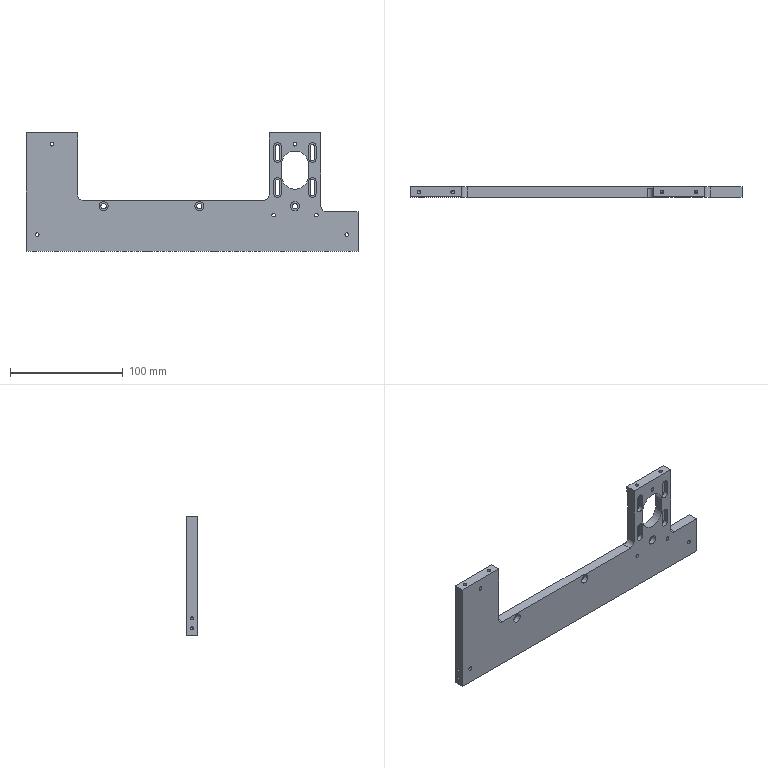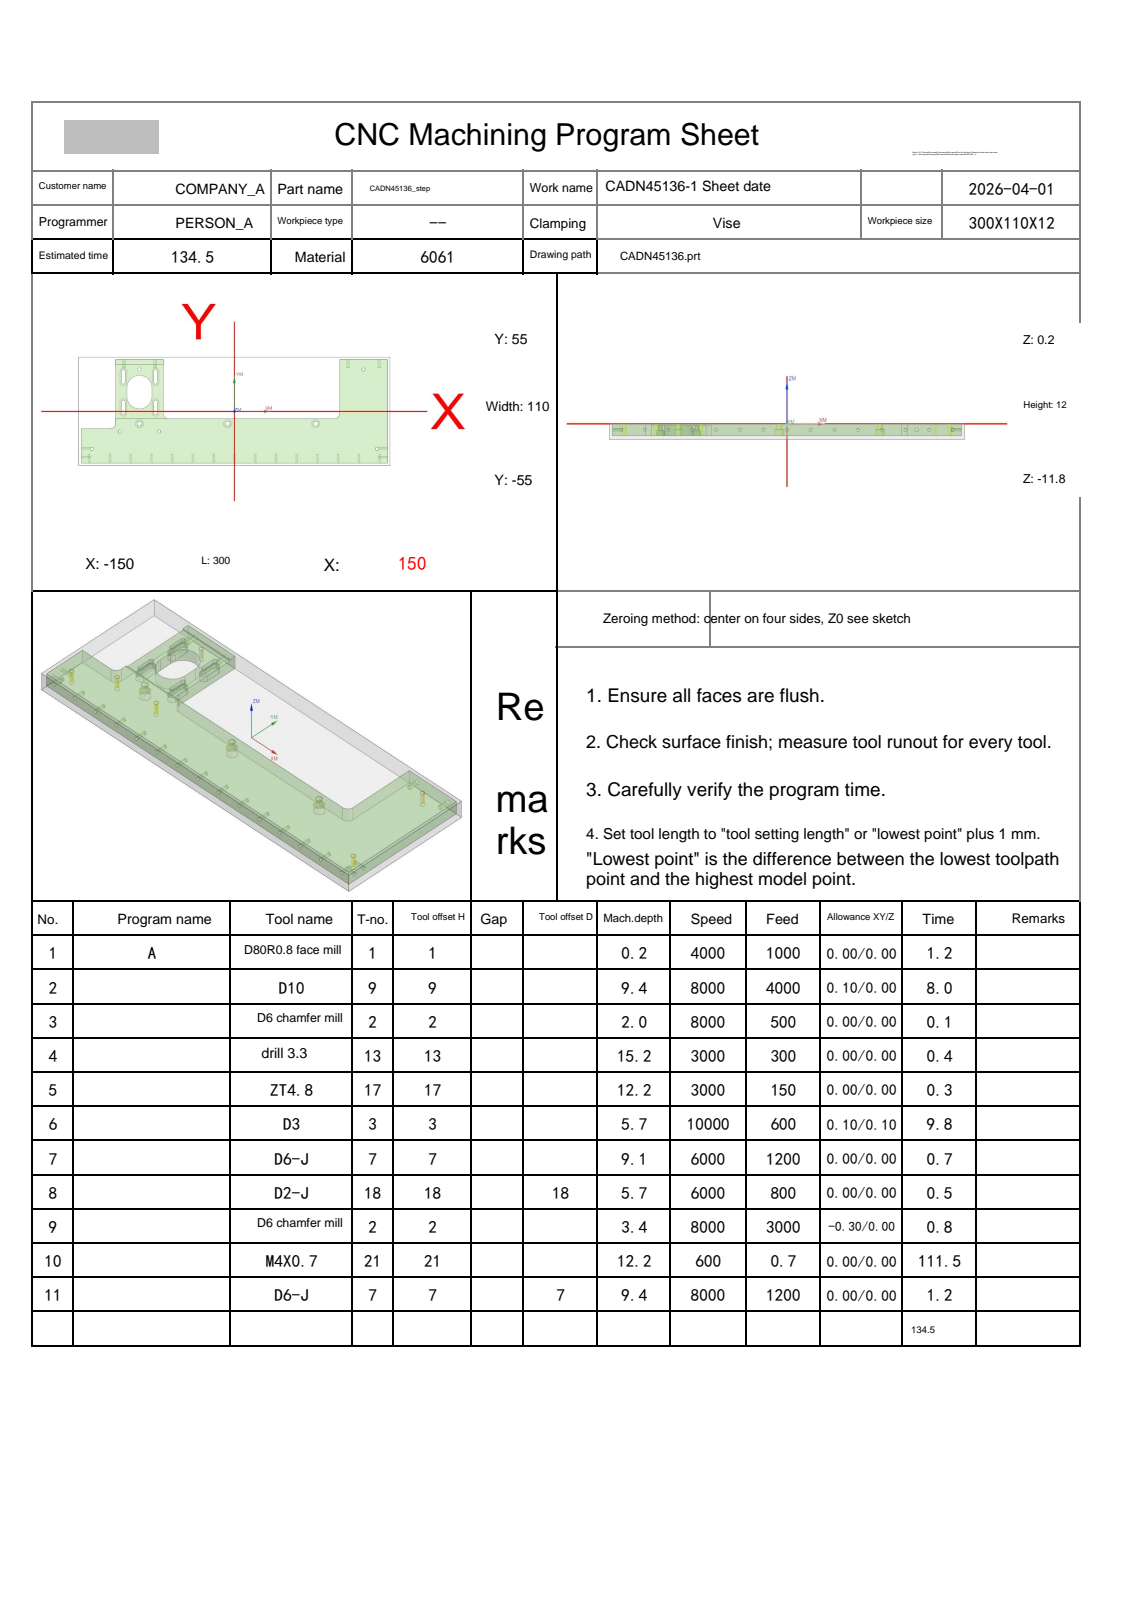NC program | NX | posted by the shop | part box 295 x 9 x 105 mm
Lines 40 to 820 of 7463:
N2 T09 M06
(D10  D=10. R=0. H=09 ce=0.25 di=0.10)
G00 G90 G54 X-68.786 Y65.963 M03 S8000
G43 H09 Z20.
M08
Z-7.2
G01 X-68.771 Y65.864 Z-7.825 F4000.
X-68.756 Y65.765 Z-8.072
X-68.741 Y65.666 Z-8.254
X-68.727 Y65.567 Z-8.4
X-68.712 Y65.468 Z-8.523
X-68.697 Y65.369 Z-8.628
X-68.683 Y65.271 Z-8.72
X-68.668 Y65.172 Z-8.8
X-68.653 Y65.073 Z-8.87
X-68.638 Y64.974 Z-8.932
X-68.624 Y64.875 Z-8.986
X-68.609 Y64.776 Z-9.033
X-68.594 Y64.677 Z-9.074
X-68.579 Y64.578 Z-9.108
X-68.565 Y64.479 Z-9.136
X-68.55 Y64.38 Z-9.16
X-68.535 Y64.281 Z-9.177
X-68.52 Y64.183 Z-9.19
X-68.506 Y64.084 Z-9.197
X-68.491 Y63.985 Z-9.2
X-68.183 Y61.92
G03 X-67.828 Y61.51 I.503 J.077
X-64.07 Y61.003 I3.766 J13.735
X-55.015 Y60.895 I9.055 J380.264
X-53.111 Y60.9 I0.0 J380.372
G01 X148.548 Y60.876
G02 X154.516 Y56.713 I-.244 J-6.709
X155.74 Y50.873 I-15.367 J-6.267
X155.919 Y41.406 I-249.458 J-9.468
X155.9 Y38.276 I-249.637 J0.0
G01 X155.881 Y-53.443
G02 X151.609 Y-59.576 I-6.76 J.154
X145.818 Y-60.747 I-6.194 J15.737
X136.002 Y-60.92 I-9.816 J277.475
X132.62 Y-60.9 I0.0 J277.648
G01 X-148.443 Y-60.881
G02 X-154.576 Y-56.609 I.154 J6.761
X-155.75 Y-50.758 I15.84 J6.222
X-155.919 Y-40.968 I283.441 J9.79
X-155.9 Y-37.62 I283.61 J0.0
G01 X-155.881 Y53.463
G02 X-151.482 Y59.632 I6.792 J-.189
X-145.858 Y60.744 I6.093 J-16.036
X-136.388 Y60.919 I9.47 J-257.302
X-133.261 Y60.9 I0.0 J-257.476
G01 X-70.041 Y60.879
G03 X-57.209 Y60.291 I12.832 J139.682
X-55.325 Y60.304 I0.0 J140.271
G01 X146.849 Y60.277
G02 X153.44 Y55.91 I-.376 J-7.725
X155.033 Y49.733 I-14.85 J-7.123
X155.315 Y40.999 I-135.175 J-8.734
X155.297 Y38.82 I-135.457 J0.0
G01 X155.276 Y-51.847
G02 X150.921 Y-58.441 I-7.715 J.36
X144.799 Y-60.029 I-7.08 J14.703
X136.255 Y-60.312 I-8.544 J128.757
X134.246 Y-60.297 I0.0 J129.04
G01 X-146.788 Y-60.279
G02 X-153.493 Y-55.822 I.313 J7.744
X-155.023 Y-49.865 I14.84 J6.985
X-155.302 Y-41.99 I110.955 J7.875
X-155.294 Y-40.632 I111.234 J0.0
G01 X-155.279 Y51.788
G02 X-150.981 Y58.41 I7.703 J-.294
X-144.864 Y60.023 I7.093 J-14.49
X-136.955 Y60.303 I7.909 J-111.65
X-135.571 Y60.294 I0.0 J-111.93
G01 X-71.631 Y60.284
G03 X-62.812 Y59.814 I57.469 J996.395
X-51.581 Y59.699 I11.231 J545.885
X-50.111 Y59.701 I0.0 J546.001
G01 X145.169 Y59.68
G02 X152.839 Y54.507 I-.295 J-8.712
X154.414 Y48.069 I-16.783 J-7.517
X154.705 Y39.47 I-126.982 J-8.599
X154.694 Y37.816 I-127.273 J0.0
G01 X154.675 Y-50.243
G02 X149.608 Y-57.796 I-8.677 J.345
X143.065 Y-59.417 I-7.586 J16.605
X133.778 Y-59.715 I-9.287 J144.477
X131.492 Y-59.697 I0.0 J144.775
G01 X-145.208 Y-59.677
G02 X-152.851 Y-54.498 I.321 J8.702
X-154.412 Y-48.122 I16.765 J7.484
X-154.706 Y-39.479 I126.879 J8.643
X-154.695 Y-37.809 I127.173 J0.0
G01 X-154.675 Y50.251
G02 X-149.622 Y57.786 I8.675 J-.355
X-143.195 Y59.404 I7.576 J-16.526
X-134.131 Y59.712 I9.064 J-132.923
X-132.042 Y59.696 I0.0 J-133.231
G01 X-72.722 Y59.682
G02 X-63.107 Y59.239 I-33.813 J-837.622
G03 X-51.393 Y59.1 I11.714 J493.752
X-50.11 Y59.101 I0.0 J493.891
G01 X143.669 Y59.077
G02 X148.675 Y57.598 I-.315 J-10.277
X150.125 Y57.047 I-1.928 J-7.251
G01 X151.212 Y56.212
X152.047 Y55.125
G02 X153.419 Y50.239 I-16.938 J-7.393
X154.07 Y41.14 I-63.251 J-9.099
X154.067 Y40.491 I-63.902 J0.0
G01 X154.099 Y30.351
X154.076 Y-48.649
G02 X152.605 Y-53.654 I-9.869 J.182
X152.047 Y-55.125 I-7.571 J2.033
G01 X151.212 Y-56.212
X150.125 Y-57.047
G02 X145.652 Y-58.348 I-7.112 J16.105
X136.776 Y-59.053 I-8.875 J55.541
G01 X136.51 Y-59.052
X125.35 Y-59.099
X-143.67 Y-59.075
G02 X-148.676 Y-57.599 I.237 J10.028
X-150.125 Y-57.047 I2.048 J7.549
G01 X-151.212 Y-56.212
X-152.047 Y-55.125
G02 X-153.391 Y-50.416 I16.58 J7.279
X-154.066 Y-41.352 I60.501 J9.065
X-154.063 Y-40.79 I61.176 J0.0
G01 X-154.098 Y-31.671
X-154.076 Y48.649
G02 X-148.384 Y57.183 I9.462 J-.146
X-141.53 Y58.809 I8.014 J-18.516
X-132.244 Y59.109 I9.286 J-143.8
X-130.257 Y59.095 I0.0 J-144.1
G01 X-73.577 Y59.08
G02 X-62.877 Y58.642 I-27.703 J-807.761
G03 X-50.397 Y58.5 I12.48 J549.906
X-49.15 Y58.502 I0.0 J550.047
G01 X142.169 Y58.479
G02 X146.239 Y57.75 I-.385 J-13.872
X146.807 Y57.765 I.568 J-10.591
X148.751 Y57.585 I0.0 J-10.606
G03 X146.437 Y57.771 I-2.314 J-14.306
X145.781 Y57.756 I0.0 J-14.492
X137.77 Y58.028 I-8.011 J-117.995
X136.203 Y58.018 I0.0 J-118.266
G01 X-56.084 Y58.043
G02 X-72.109 Y58.552 I6.852 J468.627
G03 X-80.688 Y58.618 I-8.844 J-591.068
G01 X-134.548 Y58.59
G03 X-135.199 Y58.593 I-.651 J-60.006
X-143.402 Y58.03 I0.0 J-60.01
X-149.644 Y55.55 I1.793 J-13.612
X-153.206 Y49.151 I6.171 J-7.625
X-153.61 Y42.924 I47.678 J-6.227
X-153.603 Y42.089 I48.083 J0.0
G01 X-153.598 Y-39.071
G03 X-153.602 Y-39.931 I77.983 J-.86
X-153.086 Y-48.891 I77.988 J0.0
G01 X-152.75 Y-50.863
G03 X-152.774 Y-51.633 I12.285 J-.77
X-152.571 Y-53.859 I12.309 J0.0
G02 X-152.774 Y-51.633 I12.106 J2.226
X-152.75 Y-50.863 I12.309 J0.0
G03 X-152.949 Y-41.559 I-232.624 J-.324
G02 X-153.024 Y-31.151 I719.15 J10.408
X-153.018 Y-28.119 I719.225 J0.0
G01 X-152.994 Y42.301
G02 X-153. Y42.949 I35.009 J.649
X-152.496 Y48.871 I35.015 J0.0
X-146.142 Y56.306 I9.945 J-2.067
X-138.997 Y57.773 I8.169 J-21.648
X-129.006 Y58.032 I9.991 J-192.317
X-126.522 Y58.016 I0.0 J-192.577
G01 X-75.182 Y57.996
G02 X-61.404 Y57.536 I-23.436 J-909.651
G03 X-48.423 Y57.418 I12.981 J712.896
X-46.331 Y57.421 I0.0 J713.014
G01 X99.827 Y57.444
X100.141 Y57.571
X101.502 Y57.75
X145.962
G03 X146.462 Y58.25 I0.0 J.5
X146.23 Y58.672 I-.5 J0.0
G01 X145.472 Y59.154
X143.803 Y60.216 Z-9.1
X143.471 Y60.426
X143.41 Y60.46
X143.345 Y60.484
X143.277 Y60.499
X143.207 Y60.504
X101.792 Y60.822
X101.709 Y60.816
X101.628 Y60.795
X101.551 Y60.762
X101.481 Y60.717
X101.42 Y60.66
X101.369 Y60.594
X101.329 Y60.521
X101.202 Y60.227
X100.415 Y58.412 Z-9.2
X100.076 Y57.643
G02 X99.194 Y57.273 I-.934 J.987
X94.052 Y56.951 I-5.142 J40.964
X93.238 Y56.959 I0.0 J41.286
G01 X-54.412 Y56.957
G02 X-66.375 Y57.254 I1.4 J298.37
G01 X-67.141 Y57.571
X-68.498 Y57.75
X-114.559 Y57.742
G02 X-121.715 Y57.521 I-7.155 J115.808
X-123.687 Y57.538 I0.0 J116.029
G03 X-126.982 Y57.558 I-3.295 J-268.593
X-137.903 Y57.336 I0.0 J-268.613
X-145.133 Y56.003 I.793 J-24.574
X-151.833 Y48.166 I3.59 J-9.852
X-152.494 Y41.412 I34.197 J-6.754
X-152.493 Y41.13 I34.857 J0.0
G01 X-152.538 Y31.59
X-152.56 Y-16.114
X-152.75 Y-17.498
Y-47.858
G02 X-153.25 Y-48.358 I-.5 J0.0
X-153.672 Y-48.126 I0.0 J.5
G01 X-154.155 Y-47.366
X-155.216 Y-45.696 Z-9.1
X-155.427 Y-45.364
X-155.46 Y-45.303
X-155.484 Y-45.239
X-155.499 Y-45.172
X-155.505 Y-45.104
X-155.934 Y-18.062
X-155.928 Y-17.978
X-155.908 Y-17.896
X-155.875 Y-17.819
X-155.829 Y-17.748
X-155.772 Y-17.686
X-155.706 Y-17.635
X-155.632 Y-17.595
X-155.242 Y-17.426
X-153.425 Y-16.642 Z-9.2
X-152.755 Y-16.346
G03 X-152.322 Y-15.277 I-1.299 J1.149
X-151.955 Y-9.758 I-41.263 J5.519
X-151.962 Y-9.007 I-41.63 J0.0
G01 X-151.911 Y39.449
G02 X-151.915 Y40.07 I41.231 J.621
X-151.343 Y46.917 I41.235 J0.0
X-144.116 Y55.353 I10.759 J-1.903
X-136.649 Y56.725 I8.369 J-24.555
X-125.37 Y56.959 I11.279 J-271.073
X-122.371 Y56.942 I0.0 J-271.308
G03 X-121.606 Y56.939 I.764 J93.639
X-117.125 Y57.047 I0.0 J93.642
G01 X-115.859 Y57.571
X-114.55 Y57.743
X-115.859 Y57.571
G02 X-119.804 Y56.605 I-4.069 J8.073
X-130.792 Y56.413 I-10.988 J314.503
G01 X-131.508
X-131.837 Y56.414
G03 X-140.295 Y55.769 I0.0 J-55.728
X-146.815 Y53.03 I2.081 J-14.085
X-150.712 Y46.343 I7.555 J-8.882
X-151.412 Y39.014 I38.02 J-7.329
X-151.411 Y38.708 I38.72 J0.0
G01 X-151.458 Y28.808
X-151.485 Y-8.765
G02 X-151.481 Y-9.31 I-40.224 J-.545
X-151.821 Y-14.533 I-40.228 J0.0
G03 X-152.506 Y-15.984 I4.769 J-3.138
G02 X-151.728 Y-14.401 I5.56 J-1.751
G03 X-151.04 Y-10.594 I-11.607 J4.064
X-150.851 Y-2.255 I-183.773 J8.339
X-150.859 Y-.53 I-183.962 J0.0
G01 X-150.832 Y36.809
G02 X-150.837 Y37.511 I48.195 J.702
X-150.261 Y44.939 I48.2 J0.0
X-146.631 Y51.841 I11.812 J-1.807
X-139.977 Y54.993 I9.229 J-10.884
X-131.236 Y55.792 I8.741 J-47.384
G01 X-131.146
G03 X-120.479 Y56.007 I-.823 J305.744
X-117.968 Y56.4 I-.168 J9.294
G01 X-117.125 Y57.047
G02 X-119.928 Y55.776 I-3.254 J3.449
X-126.122 Y55.388 I-6.194 J49.27
X-126.459 Y55.389 I0.0 J49.658
G03 X-126.977 Y55.39 I-.518 J-111.012
X-136.698 Y54.964 I0.0 J-111.013
X-143.704 Y53.001 I1.554 J-19.027
X-149.377 Y45.566 I5.649 J-10.193
X-150.291 Y38.08 I31.407 J-7.633
X-150.378 Y27.767 I609.102 J-10.313
G01 Y26.86
X-150.403 Y-5.23
G02 X-150.398 Y-5.905 I-49.547 J-.675
X-150.828 Y-12.419 I-49.552 J0.0
X-151.212 Y-13.788 I-4.983 J.66
G01 X-151.87 Y-14.645
G03 X-150.747 Y-12.973 I-5.022 J4.588
X-149.95 Y-8.12 I-16.475 J5.196
X-149.765 Y1.489 I-248.778 J9.609
X-149.778 Y4.089 I-248.964 J0.0
G01 X-149.748 Y34.849
G02 X-149.752 Y35.499 I50.631 J.65
X-149.142 Y43.337 I50.635 J0.0
X-145.752 Y50.231 I12.711 J-1.969
X-138.839 Y53.806 I9.685 J-10.257
X-130.019 Y54.701 I8.98 J-44.607
G03 X-121.432 Y55.052 I-.675 J121.785
X-118.603 Y55.728 I-.487 J8.287
G02 X-117.974 Y56.395 I2.464 J-1.694
G03 X-118.614 Y55.697 I1.576 J-2.088
G02 X-121.316 Y54.754 I-3.37 J5.308
X-128.025 Y54.283 I-7.13 J53.574
G03 X-136.933 Y53.617 I.376 J-64.906
X-143.797 Y50.919 I2.195 J-15.669
X-148.345 Y43.737 I7.694 J-9.903
X-149.217 Y35.941 I35.474 J-7.913
X-149.297 Y25.914 I621.652 J-10.028
G01 Y25.622
X-149.325 Y-2.828
G02 X-149.321 Y-3.477 I-55.604 J-.648
X-149.792 Y-10.702 I-55.608 J0.0
X-150.65 Y-13.348 I-7.16 J.858
G01 X-151.205 Y-13.782
G03 X-149.699 Y-11.683 I-1.87 J2.932
X-148.861 Y-5.993 I-21.722 J6.106
X-148.684 Y4.381 I-305.289 J10.374
X-148.698 Y7.269 I-305.465 J0.0
G01 X-148.668 Y32.809
G02 X-148.672 Y33.485 I54.884 J.676
X-148.061 Y41.658 I54.888 J0.0
X-144.879 Y48.622 I13.632 J-2.018
X-137.852 Y52.591 I10.07 J-9.624
X-129.468 Y53.604 I9.193 J-40.884
G03 X-121.979 Y54.13 I-1.305 J72.255
X-119.154 Y54.999 I-.943 J8.088
G01 X-118.572 Y55.744
G02 X-119.554 Y54.67 I-3.103 J1.85
X-123.255 Y53.599 I-4.607 J8.991
X-130.947 Y53.035 I-12.623 J119.535
G03 X-138.788 Y51.686 I1.192 J-30.378
X-147.067 Y42.897 I3.873 J-11.942
X-148.097 Y35.245 I31.408 J-8.123
X-148.226 Y24.802 I424.702 J-10.443
X-148.218 Y22.226 I424.83 J0.0
G01 X-148.248 Y-.905
G02 X-148.244 Y-1.559 I-58.96 J-.654
X-148.78 Y-9.488 I-58.964 J0.0
X-149.931 Y-12.826 I-8.323 J1.003
G01 X-150.601 Y-13.319
G03 X-149.613 Y-12.538 I-3.219 J5.094
X-148.285 Y-9.065 I-6.834 J4.603
X-147.671 Y-1.149 I-50.739 J7.916
G01 Y-.93
X-147.618 Y9.309
X-147.589 Y30.809
G02 X-147.593 Y31.447 I61.772 J.638
X-147.028 Y39.783 I61.776 J0.0
X-144.168 Y46.821 I14.934 J-1.968
X-137.126 Y51.308 I10.493 J-8.698
X-129.132 Y52.509 I9.654 J-37.075
G03 X-122.251 Y53.253 I-2.097 J51.6
X-119.385 Y54.43 I-1.105 J6.767
X-119.047 Y55.125 I-2.527 J1.662
G02 X-120.426 Y53.615 I-2.203 J.628
X-125.058 Y52.432 I-5.836 J13.182
G03 X-132.691 Y51.659 I52.124 J-553.045
X-139.938 Y49.455 I2.129 J-20.019
X-145.982 Y41.424 I6.51 J-11.19
X-147.031 Y33.17 I34.13 J-8.53
X-147.139 Y22.944 I486.902 J-10.226
X-147.137 Y21.831 I487.009 J0.0
G01 X-147.168 Y1.013
G02 X-147.164 Y.337 I-65.753 J-.676
X-147.728 Y-8.252 I-65.757 J0.0
X-149.106 Y-12.263 I-9.883 J1.154
X-150.025 Y-12.912 I-1.278 J.835
G03 X-148.319 Y-11.362 I-.853 J2.653
X-147.013 Y-6.549 I-12.819 J6.062
X-146.552 Y2.684 I-92.147 J9.233
X-146.556 Y3.578 I-92.609 J0.0
G01 X-146.499 Y29.789
G02 X-146.502 Y30.295 I55.704 J.506
X-145.837 Y38.874 I55.706 J0.0
X-142.562 Y46.118 I14.6 J-2.238
X-135.397 Y50.326 I10.589 J-9.827
X-128.536 Y51.453 I10.344 J-41.506
G03 X-122.21 Y52.459 I-2.581 J36.644
X-119.615 Y53.792 I-1.442 J5.999
G01 X-119.293 Y54.531
G02 X-120.933 Y52.701 I-2.73 J.796
X-125.878 Y51.343 I-6.657 J14.559
G03 X-133.252 Y50.271 I14.392 J-124.874
X-140.401 Y47.159 I2.877 J-16.377
X-144.992 Y39.65 I8.849 J-10.568
X-145.952 Y31.503 I37.313 J-8.529
X-146.08 Y16.182 I919.511 J-15.321
X-146.058 Y9.78 I919.639 J0.0
G02 X-146.039 Y6.984 I-211.212 J-2.796
X-146.331 Y-4.12 I-211.23 J0.0
X-147.448 Y-10.224 I-22.607 J.98
X-148.798 Y-12.398 I-5.143 J1.689
G01 X-149.469 Y-12.681
G03 X-147.472 Y-10.969 I-.887 J3.055
X-146.002 Y-5.848 I-13.124 J6.538
X-145.476 Y3.866 I-89.448 J9.715
X-145.48 Y4.723 I-89.974 J0.0
G01 X-145.414 Y28.429
G02 X-145.416 Y28.778 I56.791 J.349
X-144.758 Y37.395 I56.792 J0.0
X-141.557 Y44.736 I15.216 J-2.266
X-134.413 Y49.158 I10.938 J-9.689
X-127.47 Y50.502 I12.756 J-47.298
G03 X-121.744 Y51.854 I-2.689 J24.198
X-119.665 Y53.332 I-1.53 J4.354
G01 X-119.571 Y53.859
G02 X-120.31 Y52.481 I-1.729 J.04
X-124.123 Y50.746 I-5.788 J7.663
X-130.778 Y49.482 I-24.756 J112.188
G03 X-137.811 Y46.997 I3.305 J-20.547
X-143.738 Y38.883 I7.252 J-11.519
X-144.848 Y30.577 I34.334 J-8.814
X-144.999 Y16.886 I618.318 J-13.691
X-144.978 Y11.699 I618.47 J0.0
G02 X-144.959 Y8.781 I-229.843 J-2.919
X-145.249 Y-2.756 I-229.862 J0.0
X-146.448 Y-9.53 I-25.415 J1.007
X-148.269 Y-12.295 I-5.566 J1.684
X-148.859 Y-12.429 I-.749 J1.93
G03 X-147.196 Y-11.483 I-.135 J2.172
X-145.346 Y-7.177 I-8.291 J6.114
X-144.491 Y1.349 I-46.779 J8.996
X-144.352 Y17.57 I-948.957 J16.22
X-144.368 Y23.029 I-949.096 J0.0
G02 X-144.379 Y24.56 I106.277 J1.531
X-143.948 Y34.116 I106.288 J0.0
X-141.754 Y41.608 I19.558 J-1.659
X-134.263 Y47.724 I11.992 J-7.043
X-127.432 Y49.436 I13.717 J-40.26
G03 X-121.834 Y51.049 I-3.651 J23.179
X-119.739 Y52.719 I-1.912 J4.548
G01 X-119.63 Y53.412
G02 X-120.597 Y51.582 I-2.25 J.019
X-124.807 Y49.631 I-6.746 J9.04
X-130.979 Y48.173 I-147.189 J609.401
G03 X-137.925 Y44.963 I4.014 J-17.804
X-142.797 Y37.01 I9.222 J-11.119
X-143.8 Y28.144 I40.502 J-9.073
X-143.923 Y13.22 I907.47 J-14.924
X-143.909 Y8.124 I907.593 J0.0
G02 X-143.901 Y6.809 I-119.703 J-1.314
X-144.376 Y-3.842 I-119.71 J0.0
X-145.855 Y-9.904 I-19.653 J1.583
X-147.765 Y-12.264 I-4.823 J1.951
G01 X-148.412 Y-12.37
G03 X-146.36 Y-11.25 I-.098 J2.62
X-144.356 Y-6.668 I-8.908 J6.625
X-143.436 Y1.911 I-46.418 J9.318
X-143.274 Y16.918 I-695.746 J15.007
X-143.288 Y21.351 I-695.908 J0.0
G02 X-143.297 Y22.81 I116.206 J1.459
X-142.902 Y32.38 I116.215 J0.0
X-140.856 Y39.989 I21.078 J-1.59
X-133.395 Y46.546 I12.51 J-6.71
X-126.834 Y48.495 I16.726 J-44.296
G03 X-121.584 Y50.407 I-4.212 J19.723
X-119.766 Y52.145 I-1.961 J3.871
G01 X-119.711 Y52.799
G02 X-119.815 Y51.942 I-4.444 J.104
X-121.897 Y49.925 I-4.251 J2.306
X-126.947 Y48.026 I-10.142 J19.3
G03 X-133.458 Y45.884 I9.861 J-40.935
X-141.601 Y36.117 I5.88 J-13.18
X-142.694 Y27.444 I37.617 J-9.146
X-142.845 Y11.781 I810.55 J-15.663
X-142.837 Y8.255 I810.701 J0.0
G02 X-142.833 Y7.265 I-105.286 J-.99
X-143.4 Y-3.655 I-105.291 J0.0
X-145.033 Y-9.763 I-19.253 J1.875
X-147.177 Y-12.221 I-4.892 J2.103
G01 X-147.796 Y-12.289
X-147.774
G03 X-145.723 Y-11.294 I0.0 J2.611
X-143.514 Y-6.801 I-8.171 J6.808
X-142.422 Y1.551 I-40.179 J9.496
X-142.193 Y15.565 I-428.131 J14.014
X-142.21 Y19.334 I-428.36 J0.0
G02 X-142.221 Y20.992 I126.283 J1.659
X-141.831 Y30.903 I126.294 J0.0
X-139.795 Y38.695 I21.991 J-1.585
X-132.368 Y45.472 I13.03 J-6.821
X-126.034 Y47.661 I22.691 J-55.391
G03 X-121.171 Y49.902 I-4.486 J16.132
X-119.754 Y51.574 I-2.034 J3.159
G01 X-119.75 Y52.209
G02 X-119.733 Y51.936 I-2.249 J-.273
X-120.499 Y50.238 I-2.265 J0.0
X-124.345 Y47.862 I-7.43 J7.727
X-130.417 Y45.699 I-247.317 J684.447
G03 X-137.239 Y41.201 I5.648 J-15.988
X-140.862 Y33.379 I12.775 J-10.668
X-141.671 Y24.07 I53.116 J-9.309
G01 Y24.007
X-141.802 Y6.145
Y6.127
G02 X-142.598 Y-4.545 I-71.998 J0.0
X-144.594 Y-10.318 I-15.786 J2.23
X-146.674 Y-12.241 I-4.017 J2.256
G01 X-147.275 Y-12.25
G03 X-147.04 Y-12.261 I.236 J2.55
X-145.125 Y-11.4 I0.0 J2.561
X-142.71 Y-7.037 I-7.4 J6.944
X-141.403 Y1.539 I-36.185 J9.906
X-141.119 Y14.448 I-293.745 J12.909
X-141.132 Y17.219 I-294.028 J0.0
G02 X-141.145 Y19.085 I140.538 J1.866
X-140.766 Y29.389 I140.551 J0.0
X-138.785 Y37.326 I23.154 J-1.565
X-131.626 Y44.306 I13.585 J-6.773
X-125.286 Y46.876 I31.591 J-68.809
G03 X-120.83 Y49.386 I-4.835 J13.795
X-119.75 Y50.888 I-2.085 J2.64
G01 Y51.608
G02 X-119.727 Y51.266 I-2.519 J-.341
X-120.519 Y49.422 I-2.542 J0.0
X-124.33 Y46.872 I-8.18 J8.101
G03 X-130.37 Y44.314 I146. J-353.157
X-137.33 Y38.481 I6.514 J-14.843
X-140.035 Y30.647 I16.853 J-10.201
X-140.627 Y21.091 I76.812 J-9.556
X-140.625 Y20.532 I77.404 J0.0
G02 X-140.622 Y18.912 I-548.823 J-1.619
X-140.841 Y3.433 I-548.826 J0.0
X-141.986 Y-5.933 I-47.274 J1.026
X-144.321 Y-10.962 I-12.371 J2.689
X-146.074 Y-12.25 I-3.04 J2.3
G01 X-146.734
G03 X-146.413 Y-12.268 I.32 J2.789
X-144.331 Y-11.344 I0.0 J2.808
X-141.796 Y-6.906 I-7.602 J7.286
X-140.369 Y1.81 I-35.491 J10.284
X-140.041 Y14.788 I-256.256 J12.977
X-140.05 Y16.947 I-256.585 J0.0
G02 X-140.058 Y18.364 I123.967 J1.417
X-139.646 Y28.455 I123.975 J0.0
X-137.535 Y36.477 I22.814 J-1.717
X-130.532 Y43.36 I14.217 J-7.46
X-124.541 Y46.151 I57.198 J-114.95
G03 X-120.541 Y48.845 I-5.186 J12.018
X-119.75 Y50.108 I-2.223 J2.273
G01 Y50.828
G02 X-119.729 Y50.495 I-2.703 J-.333
X-120.547 Y48.549 I-2.723 J0.0
X-124.363 Y45.817 I-9.1 J8.674
G03 X-130.23 Y42.908 I59.451 J-127.288
X-138.486 Y31.834 I7.793 J-14.425
X-139.483 Y22.363 I46.51 J-9.684
X-139.64 Y8.541 I943.895 J-17.613
G02 X-140.44 Y-2.931 I-83.628 J.075
X-142.551 Y-9.551 I-19.449 J2.553
X-145.17 Y-12.199 I-5.48 J2.801
X-145.759 Y-12.263 I-.589 J2.674
X-146.024 Y-12.25 I0.0 J2.738
G03 X-145.705 Y-12.267 I.319 J2.928
X-143.539 Y-11.318 I0.0 J2.945
X-140.859 Y-6.739 I-7.808 J7.645
X-139.357 Y1.797 I-34.577 J10.483
X-138.965 Y14.764 I-214.049 J12.967
X-138.97 Y16.237 I-214.442 J0.0
G02 X-138.976 Y17.441 I112.572 J1.205
X-138.509 Y27.682 I112.578 J0.0
X-136.192 Y35.829 I22.215 J-1.917
X-129.502 Y42.44 I14.938 J-8.425
X-123.822 Y45.472 I201.446 J-370.549
G03 X-120.207 Y48.393 I-5.256 J10.2
X-119.75 Y49.271 I-2.33 J1.772
G01 Y50.051
G02 X-119.729 Y49.697 I-2.95 J-.355
X-120.614 Y47.581 I-2.971 J0.0
X-124.559 Y44.614 I-10.57 J9.949
G03 X-130.361 Y41.241 I31.92 J-61.597
X-137.409 Y30.616 I9.666 J-14.062
X-138.4 Y21.143 I47.656 J-9.775
G01 X-138.609 Y7.446
G02 X-139.64 Y-3.723 I-67.599 J.608
X-141.987 Y-9.957 I-17.349 J2.973
X-144.537 Y-12.237 I-4.893 J2.905
G01 X-145.275 Y-12.25
G03 X-144.97 Y-12.265 I.305 J3.082
X-142.684 Y-11.257 I0.0 J3.097
X-139.899 Y-6.533 I-8.194 J8.013
X-138.288 Y2.516 I-35.865 J11.051
X-137.87 Y16.516 I-234.362 J14.
X-137.872 Y17.271 I-234.78 J0.0
G02 X-137.873 Y17.8 I80.317 J.529
X-137.248 Y27.805 I80.319 J0.0
X-134.185 Y36.261 I19.913 J-2.428
X-128.135 Y41.795 I16.013 J-11.433
G03 X-122.719 Y45.119 I-61.429 J106.179
X-119.856 Y48.072 I-4.788 J7.506
G01 X-119.75 Y48.377
Y49.217
G02 X-119.726 Y48.833 I-3.14 J-.384
X-120.625 Y46.625 I-3.163 J0.0
X-124.456 Y43.518 I-11.829 J10.671
G03 X-130.037 Y39.788 I28.462 J-48.625
X-136.403 Y29.118 I11.354 J-14.007
X-137.327 Y19.696 I51.409 J-9.798
G02 X-137.649 Y5.319 I-638.324 J7.097
X-138.967 Y-4.832 I-51.275 J1.499
X-141.594 Y-10.535 I-14.8 J3.359
X-143.841 Y-12.25 I-3.898 J2.778
G01 X-144.501
G03 X-144.193 Y-12.265 I.307 J3.153
X-141.882 Y-11.264 I0.0 J3.168
X-138.98 Y-6.474 I-8.26 J8.278
X-137.303 Y2.217 I-34.434 J11.154
X-136.79 Y16.486 I-198.336 J14.268
G01 Y16.57
Y16.826
G02 X-136.111 Y26.979 I76.144 J0.0
X-132.781 Y35.708 I20.064 J-2.653
X-126.974 Y41.11 I17.866 J-13.385
G03 X-122. Y44.612 I-33.827 J53.324
X-119.765 Y47.352 I-4.701 J6.116
G01 X-119.75 Y48.342
G02 X-119.725 Y47.934 I-3.362 J-.408
X-120.584 Y45.68 I-3.386 J0.0
X-124.335 Y42.379 I-13.261 J11.287
G03 X-129.783 Y38.2 I26.332 J-39.968
X-135.339 Y27.902 I13.149 J-13.742
X-136.247 Y18.599 I53.104 J-9.877
G02 X-136.667 Y4.477 I-397.104 J4.748
X-138.21 Y-5.412 I-45.08 J1.972
X-141.018 Y-10.827 I-13.631 J3.631
X-143.039 Y-12.25 I-3.6 J2.967
G01 X-143.759
G03 X-143.41 Y-12.269 I.349 J3.241
X-141.069 Y-11.277 I0.0 J3.26
X-138.112 Y-6.569 I-8.198 J8.432
X-136.258 Y2.593 I-34.171 J11.681
X-135.706 Y16.114 I-188.939 J14.489
G02 X-134.946 Y26.336 I70.33 J-.091
X-130.842 Y35.889 I19.982 J-2.927
X-125.141 Y41.015 I23.086 J-19.941
G03 X-120.804 Y44.726 I-14.786 J21.668
X-119.75 Y46.451 I-3.648 J3.414
G01 Y47.411
G02 X-119.725 Y46.972 I-3.85 J-.438
X-119.906 Y45.803 I-3.875 J0.0
X-122.377 Y42.711 I-8.305 J4.105
X-127.302 Y38.677 I-449.313 J543.589
G03 X-134.382 Y26.174 I13.167 J-15.711
X-135.203 Y16.498 I63.179 J-10.231
G02 X-135.782 Y2.805 I-208.467 J1.96
X-137.647 Y-6.451 I-36.88 J2.617
X-140.728 Y-11.364 I-11.513 J3.797
X-142.216 Y-12.25 I-2.841 J3.08
G01 X-142.936
G03 X-142.59 Y-12.268 I.346 J3.288
X-140.243 Y-11.29 I0.0 J3.307
X-137.205 Y-6.571 I-8.195 J8.613
X-135.251 Y2.573 I-33.634 J11.966
X-134.608 Y16.14 I-185.598 J15.591
G02 X-133.678 Y26.224 I60.239 J-.474
X-126.555 Y38.372 I20.648 J-3.945
G03 X-121.843 Y42.483 I-89.331 J107.142
X-119.762 Y45.315 I-5.915 J6.525
G01 X-119.75 Y46.412
G02 X-119.729 Y45.955 I-4.984 J-.457
X-119.836 Y44.924 I-5.005 J0.0
X-121.93 Y41.924 I-7.878 J3.269
X-126.547 Y37.689 I-161.193 J171.082
G03 X-133.312 Y25.046 I14.734 J-16.015
X-134.141 Y15.31 I66.965 J-10.603
G02 X-134.829 Y2.272 I-166.131 J2.238
X-136.864 Y-6.775 I-34.513 J3.009
X-139.981 Y-11.448 I-11.092 J4.023
X-141.392 Y-12.25 I-2.659 J3.038
G01 X-142.112
G03 X-141.75 Y-12.27 I.361 J3.298
X-139.438 Y-11.331 I0.0 J3.317
X-136.307 Y-6.612 I-8.079 J8.758
X-134.246 Y2.553 I-33.119 J12.264
X-133.534 Y15.39 I-169.345 J15.823
G02 X-132.548 Y25.41 I59.956 J-.841
X-125.861 Y37.362 I21.923 J-4.419
G03 X-121.389 Y41.738 I-68.176 J74.156
X-119.75 Y44.276 I-5.272 J5.203
G01 Y45.356
G02 X-119.729 Y44.873 I-5.511 J-.483
X-119.834 Y43.801 I-5.532 J0.0
X-121.892 Y40.681 I-8.569 J3.413
G03 X-126.418 Y36.042 I561.618 J-552.477
X-132.294 Y23.661 I17.122 J-15.711
X-133.09 Y14.101 I74.754 J-11.038
G02 X-133.957 Y1.238 I-130.723 J2.352
X-136.25 Y-7.455 I-30.687 J3.443
X-139.452 Y-11.7 I-9.888 J4.129
X-140.989 Y-12.274 I-1.537 J1.773
X-141.321 Y-12.25 I0.0 J2.346
G03 X-140.94 Y-12.271 I.381 J3.469
X-138.454 Y-11.23 I0.0 J3.49
X-135.285 Y-6.356 I-8.661 J9.099
X-133.208 Y2.811 I-34.165 J12.558
X-132.442 Y15.185 I-172.473 J16.897
G02 X-131.335 Y25.01 I55.752 J-1.305
X-125.233 Y36.288 I23.249 J-5.29
G03 X-121.045 Y40.869 I-61.521 J60.442
X-119.75 Y43.09 I-5.495 J4.693
G01 Y44.23
G02 X-119.729 Y43.722 I-6.131 J-.508
X-119.831 Y42.604 I-6.152 J0.0
X-121.879 Y39.318 I-9.443 J3.604
G03 X-126.338 Y34.176 I103.169 J-93.979
X-131.26 Y22.395 I19.786 J-15.184
X-132.034 Y13.313 I81.398 J-11.512
G02 X-133.041 Y.713 I-115.743 J2.908
X-135.524 Y-7.834 I-28.873 J3.755
X-138.794 Y-11.839 I-9.21 J4.183
X-140.121 Y-12.275 I-1.327 J1.803
X-140.454 Y-12.25 I0.0 J2.239
G03 X-140.083 Y-12.269 I.371 J3.53
X-137.554 Y-11.21 I0.0 J3.549
X-134.305 Y-6.224 I-8.895 J9.347
X-132.122 Y3.462 I-35.602 J13.111
X-131.315 Y15.52 I-211.775 J20.236
G02 X-129.957 Y25.248 I48.004 J-1.744
X-124.51 Y35.318 I24.853 J-6.935
G03 X-120.749 Y39.917 I-53.037 J47.207
X-119.75 Y41.815 I-6.063 J4.403
G01 Y43.075
G02 X-119.729 Y42.519 I-7.538 J-.556
X-119.822 Y41.34 I-7.559 J0.0
X-121.775 Y37.962 I-10.235 J3.667
G03 X-126.1 Y32.327 I69.823 J-58.055
X-130.273 Y20.853 I22.875 J-14.816
X-131.106 Y10.329 I119.607 J-14.766
G02 X-132.459 Y-1.46 I-77.94 J2.969
X-135.276 Y-9.003 I-23.11 J4.334
X-138.341 Y-12.077 I-7.245 J4.158
G01 X-138.8 Y-12.25
X-139.58
G03 X-139.205 Y-12.27 I.376 J3.537
X-136.697 Y-11.235 I0.0 J3.557
X-133.4 Y-6.289 I-8.828 J9.457
X-131.118 Y3.382 I-35.145 J13.396
X-130.24 Y14.901 I-202.586 J21.234
G02 X-128.738 Y24.85 I47.705 J-2.112
X-123.733 Y34.431 I27.202 J-8.114
G03 X-120.428 Y38.985 I-42.06 J34.001
X-119.75 Y40.44 I-7.133 J4.211
G01 Y41.76
G02 X-119.73 Y41.181 I-8.583 J-.579
X-119.817 Y39.962 I-8.602 J0.0
X-121.622 Y36.569 I-11.062 J3.708
G03 X-125.751 Y30.464 I58.478 J-43.995
X-129.318 Y19.085 I26.64 J-14.6
X-130.163 Y8.54 I185.701 J-20.186
G02 X-131.858 Y-2.981 I-62.55 J3.317
X-135.006 Y-9.914 I-19.323 J4.593
X-137.824 Y-12.233 I-5.613 J3.949
G01 X-138.701 Y-12.25
G03 X-138.319 Y-12.271 I.382 J3.545
X-135.837 Y-11.265 I0.0 J3.566
X-132.513 Y-6.405 I-8.712 J9.527
X-130.167 Y2.91 I-33.948 J13.502
X-129.147 Y14.582 I-192.054 J22.664
G02 X-127.477 Y24.625 I46.579 J-2.585
X-122.958 Y33.567 I30.451 J-9.775
G03 X-120.048 Y38.178 I-29.554 J21.877
G01 X-119.75 Y38.954
Y40.394
G02 X-119.731 Y39.768 I-10.552 J-.626
X-119.811 Y38.475 I-10.57 J0.0
X-121.451 Y35.087 I-12.009 J3.724
G03 X-125.245 Y28.718 I55.414 J-37.321
X-128.342 Y17.49 I30.889 J-14.56